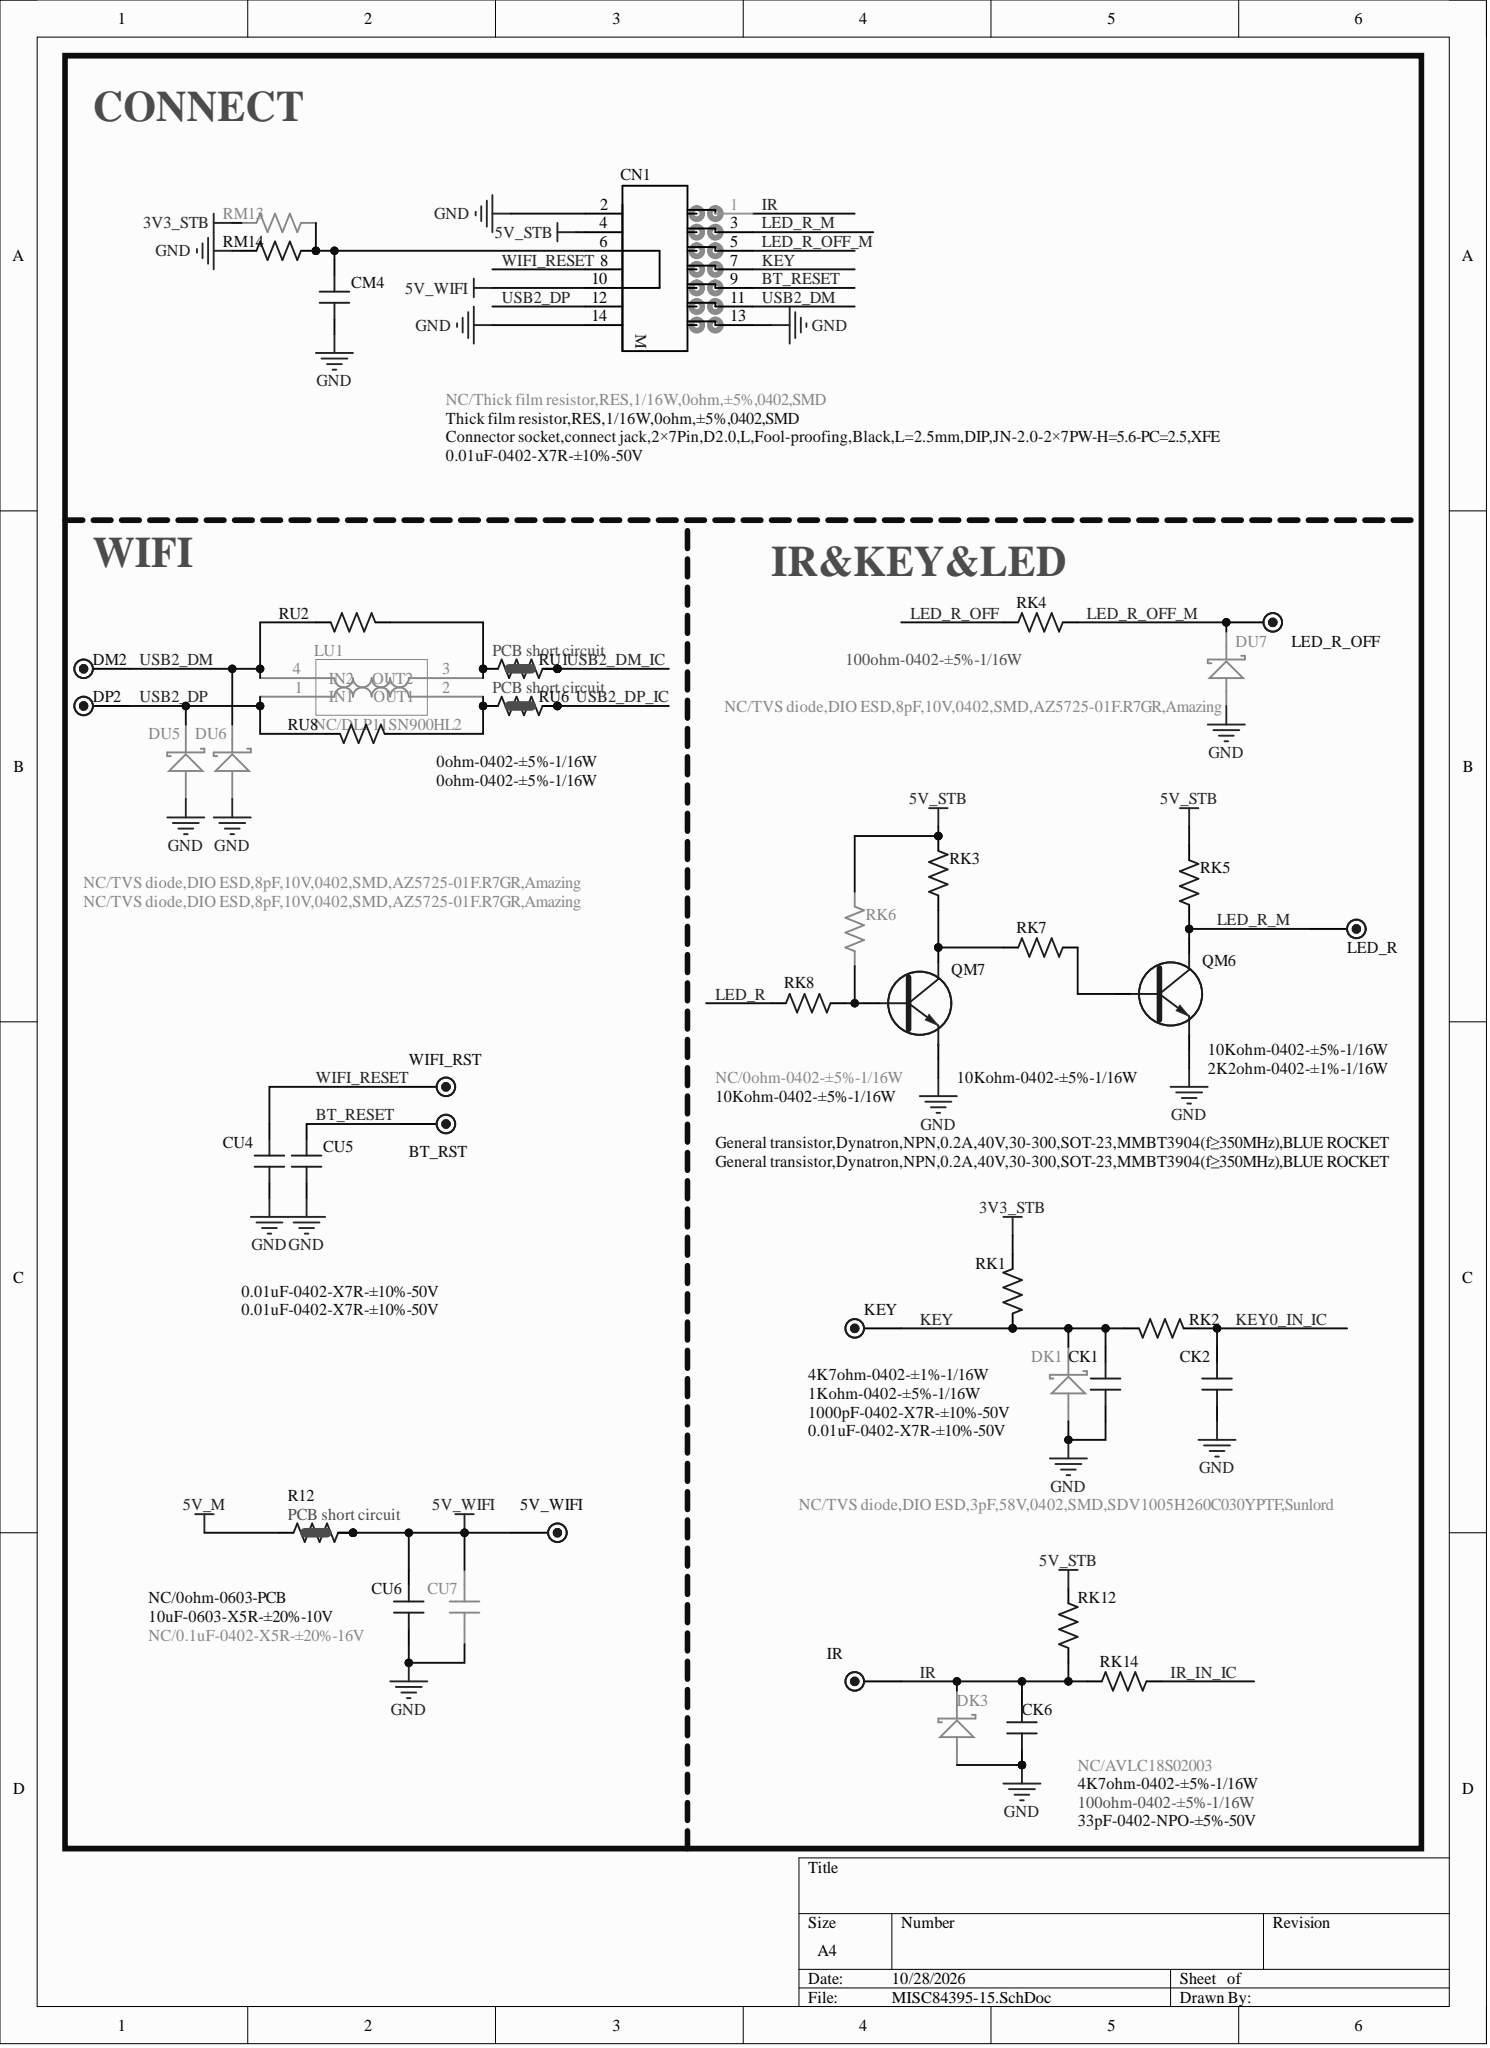Circuit board | Altium Designer | 951 parts | 509 nets | one sheet of the schematic
Parts on this sheet (reference | value | footprint):
5V_WIFI | TEST | TP
BT_RST | TEST | TP
CK1 | 1000pF-0402-X7R-±10%-50V | C0402
CK2 | 0.01uF-0402-X7R-±10%-50V | C0402
CK6 | 33pF-0402-NPO-±5%-50V | C0402
CM4 | 0.01uF-0402-X7R-±10%-50V | C0402
CN1 | Connector socket,connect jack,2×7Pin,D2.0,L,Fool-proofing,Black,L=2.5mm,DIP,JN-2.0-2×7PW-H=5.6-PC=2.5,XFE | SIP2*7H/2.0DM-8
CU4 | 0.01uF-0402-X7R-±10%-50V | C0402
CU5 | 0.01uF-0402-X7R-±10%-50V | C0402
CU6 | 10uF-0603-X5R-±20%-10V | C0603
CU7 | NC/0.1uF-0402-X5R-±20%-16V | C0402
DK1 | NC/TVS diode,DIO ESD,3pF,58V,0402,SMD,SDV1005H260C030YPTF,Sunlord | DIODE-S0402
DK3 | NC/AVLC18S02003 | DIODE-S0402
DM2 | TEST | TP
DP2 | TEST | TP
DU5 | NC/TVS diode,DIO ESD,8pF,10V,0402,SMD,AZ5725-01F.R7GR,Amazing | DIODE-S0402
DU6 | NC/TVS diode,DIO ESD,8pF,10V,0402,SMD,AZ5725-01F.R7GR,Amazing | DIODE-S0402
DU7 | NC/TVS diode,DIO ESD,8pF,10V,0402,SMD,AZ5725-01F.R7GR,Amazing | DIODE-S0402
KEY | TEST | TP
LED_R | TEST | TP
LED_R_OFF | TEST | TP
LU1 | NC/DLP11SN900HL2 | L/LC4/1.25*1.0
QM6 | General transistor,Dynatron,NPN,0.2A,40V,30-300,SOT-23,MMBT3904(f=350MHz),BLUE ROCKET | SOT-23
QM7 | General transistor,Dynatron,NPN,0.2A,40V,30-300,SOT-23,MMBT3904(f=350MHz),BLUE ROCKET | SOT-23
R12 | NC/0ohm-0603-PCB | R0603SC
RK1 | 4K7ohm-0402-±1%-1/16W | R0402
RK2 | 1Kohm-0402-±5%-1/16W | R0402
RK3 | 10Kohm-0402-±5%-1/16W | R0402
RK4 | 100ohm-0402-±5%-1/16W | R0402
RK5 | 2K2ohm-0402-±1%-1/16W | R0402
RK6 | NC/0ohm-0402-±5%-1/16W | R0402
RK7 | 10Kohm-0402-±5%-1/16W | R0402
RK8 | 10Kohm-0402-±5%-1/16W | R0402
RK12 | 4K7ohm-0402-±5%-1/16W | R0402
RK14 | 100ohm-0402-±5%-1/16W | R0402
RM13 | NC/Thick film resistor,RES,1/16W,0ohm,±5%,0402,SMD | R0402
RM14 | Thick film resistor,RES,1/16W,0ohm,±5%,0402,SMD | R0402
RU1 | NC/0ohm-0402-PCB | R0402SC
RU2 | 0ohm-0402-±5%-1/16W | R0402
RU6 | NC/0ohm-0402-PCB | R0402SC
WIFI_RST | TEST | TP
Nets of these parts (net: part-pin ...):
WIFI_RESET: CN1-8 CU4-2 WIFI_RST-1
USB2_DP_IC: RU6-2 RU6-3
USB2_DP: CN1-12 DP2-1 DU5-K LU1-1
USB2_DM_IC: RU1-2 RU1-3
USB2_DM: CN1-11 DM2-1 DU6-K LU1-4 RU2-1
NetQM7_C: QM7-C RK3-1 RK7-2
NetQM7_B: QM7-B RK6-1 RK8-2
NetQM6_B: QM6-B RK7-1
NetLU1_3: LU1-3 RU1-1 RU2-2
NetLU1_2: LU1-2 RU6-1
NetCM4_2: CM4-2 CN1-6 RM13-1 RM14-1
LED_R_OFF_M: CN1-5 DU7-K LED_R_OFF-1 RK4-2
LED_R_OFF: RK4-1
LED_R_M: CN1-3 LED_R-1 QM6-C RK5-2
LED_R: RK8-1
KEY0_IN_IC: CK2-1 RK2-1
KEY: CK1-1 CN1-7 DK1-K KEY-1 RK1-1 RK2-2
IR_IN_IC: RK14-2
IR: CK6-2 CN1-1 DK3-K RK12-1 RK14-1
GND: CK1-2 CK2-2 CK6-1 CM4-1 CN1-2 CN1-13 CN1-14 CU4-1 CU5-1 CU6-2 CU7-2 DK1-A DK3-A DU5-A DU6-A DU7-A QM6-E QM7-E RM14-2
BT_RESET: BT_RST-1 CN1-9 CU5-2
5V_WIFI: 5V_WIFI-1 CN1-10 CU6-1 CU7-1 R12-2 R12-3
5V_STB: CN1-4 RK3-2 RK5-1 RK6-2 RK12-2
5V_M: R12-1
3V3_STB: RK1-2 RM13-2